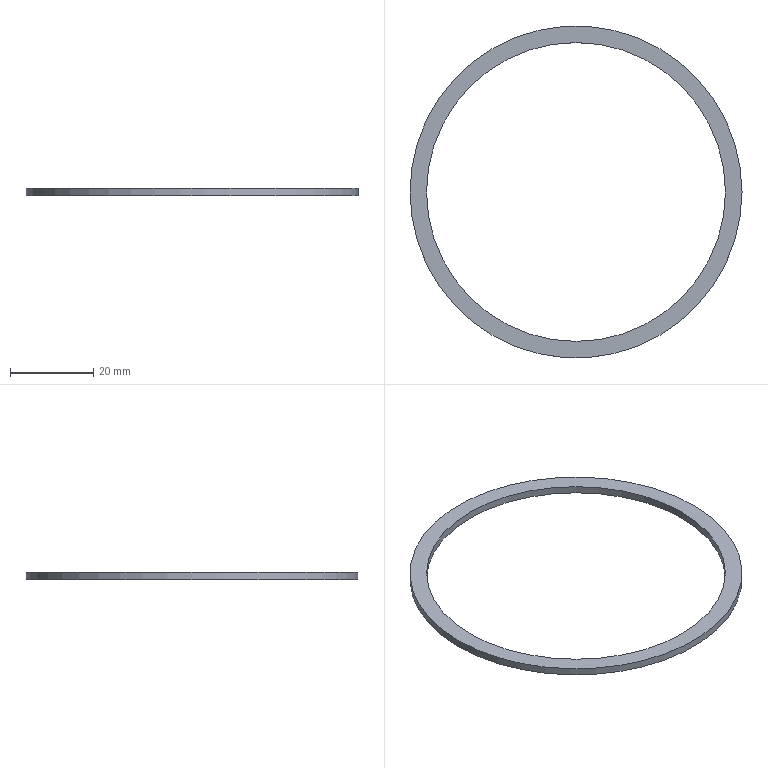Part | NX | features DATUM_CSYS 2, EXTRUDE 1, SKETCH 1 | 1 solid | 4 faces | box 80 x 80 x 1.8 mm | volume 1719 mm3 | cylinder 2 | plane 2 | commonest cylinder face diameters 72 x1 80 x1
STEP:
#1=CARTESIAN_POINT('',(40.,0.,1.8));
#2=VERTEX_POINT('',#1);
#3=CARTESIAN_POINT('',(0.,0.,1.8));
#4=DIRECTION('',(0.,0.,1.));
#5=DIRECTION('',(1.,0.,0.));
#6=AXIS2_PLACEMENT_3D('',#3,#4,#5);
#7=CIRCLE('',#6,40.);
#8=EDGE_CURVE('',#2,#2,#7,.T.);
#9=ORIENTED_EDGE('',*,*,#8,.F.);
#10=EDGE_LOOP('',(#9));
#11=FACE_BOUND('',#10,.T.);
#12=CARTESIAN_POINT('',(40.,0.,0.));
#13=VERTEX_POINT('',#12);
#14=CARTESIAN_POINT('',(0.,0.,0.));
#15=DIRECTION('',(0.,0.,1.));
#16=DIRECTION('',(1.,0.,0.));
#17=AXIS2_PLACEMENT_3D('',#14,#15,#16);
#18=CIRCLE('',#17,40.);
#19=EDGE_CURVE('',#13,#13,#18,.T.);
#20=ORIENTED_EDGE('',*,*,#19,.T.);
#21=EDGE_LOOP('',(#20));
#22=FACE_BOUND('',#21,.T.);
#23=CARTESIAN_POINT('',(0.,0.,1.8));
#24=DIRECTION('',(0.,0.,-1.));
#25=DIRECTION('',(-1.,0.,0.));
#26=AXIS2_PLACEMENT_3D('',#23,#24,#25);
#27=CYLINDRICAL_SURFACE('',#26,40.);
#28=ADVANCED_FACE('',(#11,#22),#27,.T.);
#29=CARTESIAN_POINT('',(36.,0.,1.8));
#30=VERTEX_POINT('',#29);
#31=CARTESIAN_POINT('',(0.,0.,1.8));
#32=DIRECTION('',(0.,0.,1.));
#33=DIRECTION('',(1.,0.,0.));
#34=AXIS2_PLACEMENT_3D('',#31,#32,#33);
#35=CIRCLE('',#34,36.);
#36=EDGE_CURVE('',#30,#30,#35,.T.);
#37=ORIENTED_EDGE('',*,*,#36,.T.);
#38=EDGE_LOOP('',(#37));
#39=FACE_BOUND('',#38,.T.);
#40=CARTESIAN_POINT('',(36.,0.,0.));
#41=VERTEX_POINT('',#40);
#42=CARTESIAN_POINT('',(0.,0.,0.));
#43=DIRECTION('',(0.,0.,1.));
#44=DIRECTION('',(1.,0.,0.));
#45=AXIS2_PLACEMENT_3D('',#42,#43,#44);
#46=CIRCLE('',#45,36.);
#47=EDGE_CURVE('',#41,#41,#46,.T.);
#48=ORIENTED_EDGE('',*,*,#47,.F.);
#49=EDGE_LOOP('',(#48));
#50=FACE_BOUND('',#49,.T.);
#51=CARTESIAN_POINT('',(0.,0.,1.8));
#52=DIRECTION('',(0.,0.,-1.));
#53=DIRECTION('',(-1.,0.,0.));
#54=AXIS2_PLACEMENT_3D('',#51,#52,#53);
#55=CYLINDRICAL_SURFACE('',#54,36.);
#56=ADVANCED_FACE('',(#39,#50),#55,.F.);
#57=ORIENTED_EDGE('',*,*,#8,.T.);
#58=EDGE_LOOP('',(#57));
#59=FACE_BOUND('',#58,.T.);
#60=ORIENTED_EDGE('',*,*,#36,.F.);
#61=EDGE_LOOP('',(#60));
#62=FACE_BOUND('',#61,.T.);
#63=CARTESIAN_POINT('',(0.,0.,1.8));
#64=DIRECTION('',(0.,0.,1.));
#65=DIRECTION('',(1.,0.,0.));
#66=AXIS2_PLACEMENT_3D('',#63,#64,#65);
#67=PLANE('',#66);
#68=ADVANCED_FACE('',(#59,#62),#67,.T.);
#69=ORIENTED_EDGE('',*,*,#19,.F.);
#70=EDGE_LOOP('',(#69));
#71=FACE_BOUND('',#70,.T.);
#72=ORIENTED_EDGE('',*,*,#47,.T.);
#73=EDGE_LOOP('',(#72));
#74=FACE_BOUND('',#73,.T.);
#75=CARTESIAN_POINT('',(0.,0.,0.));
#76=DIRECTION('',(0.,0.,1.));
#77=DIRECTION('',(1.,0.,0.));
#78=AXIS2_PLACEMENT_3D('',#75,#76,#77);
#79=PLANE('',#78);
#80=ADVANCED_FACE('',(#71,#74),#79,.F.);
#81=CLOSED_SHELL('',(#28,#56,#68,#80));
#82=MANIFOLD_SOLID_BREP('',#81);
#83=(LENGTH_UNIT()NAMED_UNIT(*)SI_UNIT(.MILLI.,.METRE.));
#84=UNCERTAINTY_MEASURE_WITH_UNIT(LENGTH_MEASURE(0.00001),#83,'','');
#85=(NAMED_UNIT(*)PLANE_ANGLE_UNIT()SI_UNIT($,.RADIAN.));
#86=(NAMED_UNIT(*)SI_UNIT($,.STERADIAN.)SOLID_ANGLE_UNIT());
#87=(GEOMETRIC_REPRESENTATION_CONTEXT(3)GLOBAL_UNCERTAINTY_ASSIGNED_CONTEXT((#84))GLOBAL_UNIT_ASSIGNED_CONTEXT((#83,#85,#86))REPRESENTATION_CONTEXT('',''));
#88=ADVANCED_BREP_SHAPE_REPRESENTATION('',(#82),#87);